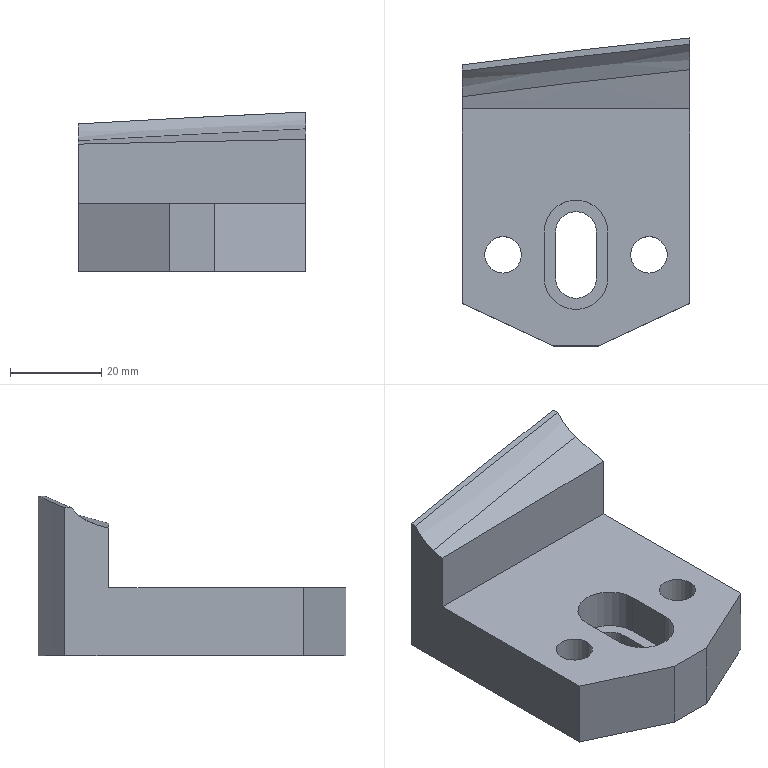Part | NX | features solid 2 | 1 solid | 23 faces | box 50 x 67.548 x 35.102 mm | volume 50758 mm3 | plane 13 | cylinder 6 | spline 4 | commonest cylinder face diameters 8 x2 9 x2 14 x2
STEP:
#1=CARTESIAN_POINT('',(-293.,-490.,-80.));
#2=VERTEX_POINT('',#1);
#3=CARTESIAN_POINT('',(-293.,-490.,-89.));
#4=VERTEX_POINT('',#3);
#5=CARTESIAN_POINT('',(-293.,-490.,-90.));
#6=DIRECTION('',(-0.000000149,0.000000502,1.));
#7=VECTOR('',#6,1000.);
#8=LINE('',#5,#7);
#9=EDGE_CURVE('',#2,#4,#8,.F.);
#10=ORIENTED_EDGE('',*,*,#9,.T.);
#11=CARTESIAN_POINT('',(-307.,-490.,-89.));
#12=VERTEX_POINT('',#11);
#13=CARTESIAN_POINT('',(-300.,-490.,-89.));
#14=DIRECTION('',(-0.000000149,0.000000502,1.));
#15=DIRECTION('',(0.,-1.,0.000000502));
#16=AXIS2_PLACEMENT_3D('',#13,#14,#15);
#17=CIRCLE('',#16,7.);
#18=EDGE_CURVE('',#12,#4,#17,.T.);
#19=ORIENTED_EDGE('',*,*,#18,.F.);
#20=CARTESIAN_POINT('',(-307.,-490.,-80.));
#21=VERTEX_POINT('',#20);
#22=CARTESIAN_POINT('',(-307.,-490.,-90.));
#23=DIRECTION('',(0.000000149,-0.000000502,-1.));
#24=VECTOR('',#23,1000.);
#25=LINE('',#22,#24);
#26=EDGE_CURVE('',#21,#12,#25,.T.);
#27=ORIENTED_EDGE('',*,*,#26,.F.);
#28=CARTESIAN_POINT('',(-300.,-490.,-80.));
#29=DIRECTION('',(0.000000149,-0.000000502,-1.));
#30=DIRECTION('',(0.,-1.,0.000000502));
#31=AXIS2_PLACEMENT_3D('',#28,#29,#30);
#32=CIRCLE('',#31,7.);
#33=EDGE_CURVE('',#2,#21,#32,.T.);
#34=ORIENTED_EDGE('',*,*,#33,.F.);
#35=EDGE_LOOP('',(#10,#19,#27,#34));
#36=FACE_BOUND('',#35,.T.);
#37=CARTESIAN_POINT('',(-300.,-490.,-90.));
#38=DIRECTION('',(0.000000149,-0.000000502,-1.));
#39=DIRECTION('',(1.,-0.000001668,0.000000149));
#40=AXIS2_PLACEMENT_3D('',#37,#38,#39);
#41=CYLINDRICAL_SURFACE('',#40,7.);
#42=ADVANCED_FACE('',(#36),#41,.F.);
#43=CARTESIAN_POINT('',(-293.,-480.,-80.));
#44=VERTEX_POINT('',#43);
#45=CARTESIAN_POINT('',(-293.,-480.,-89.));
#46=VERTEX_POINT('',#45);
#47=CARTESIAN_POINT('',(-293.,-480.,-90.));
#48=DIRECTION('',(0.000000149,-0.000000502,-1.));
#49=VECTOR('',#48,1000.);
#50=LINE('',#47,#49);
#51=EDGE_CURVE('',#44,#46,#50,.T.);
#52=ORIENTED_EDGE('',*,*,#51,.T.);
#53=CARTESIAN_POINT('',(-293.,-490.,-89.));
#54=DIRECTION('',(0.000001668,1.,-0.000000502));
#55=VECTOR('',#54,1000.);
#56=LINE('',#53,#55);
#57=EDGE_CURVE('',#4,#46,#56,.T.);
#58=ORIENTED_EDGE('',*,*,#57,.F.);
#59=ORIENTED_EDGE('',*,*,#9,.F.);
#60=CARTESIAN_POINT('',(-293.,-480.,-80.));
#61=DIRECTION('',(-0.000001668,-1.,0.000000502));
#62=VECTOR('',#61,1000.);
#63=LINE('',#60,#62);
#64=EDGE_CURVE('',#44,#2,#63,.T.);
#65=ORIENTED_EDGE('',*,*,#64,.F.);
#66=EDGE_LOOP('',(#52,#58,#59,#65));
#67=FACE_BOUND('',#66,.T.);
#68=CARTESIAN_POINT('',(-293.,-480.,-90.));
#69=DIRECTION('',(-1.,0.000001668,-0.000000149));
#70=DIRECTION('',(0.000001668,1.,-0.000000502));
#71=AXIS2_PLACEMENT_3D('',#68,#69,#70);
#72=PLANE('',#71);
#73=ADVANCED_FACE('',(#67),#72,.T.);
#74=CARTESIAN_POINT('',(-307.,-480.,-89.));
#75=VERTEX_POINT('',#74);
#76=CARTESIAN_POINT('',(-300.,-480.,-89.));
#77=DIRECTION('',(0.000000149,-0.000000502,-1.));
#78=DIRECTION('',(0.,-1.,0.000000502));
#79=AXIS2_PLACEMENT_3D('',#76,#77,#78);
#80=CIRCLE('',#79,7.);
#81=EDGE_CURVE('',#75,#46,#80,.T.);
#82=ORIENTED_EDGE('',*,*,#81,.T.);
#83=ORIENTED_EDGE('',*,*,#51,.F.);
#84=CARTESIAN_POINT('',(-307.,-480.,-80.));
#85=VERTEX_POINT('',#84);
#86=CARTESIAN_POINT('',(-300.,-480.,-80.));
#87=DIRECTION('',(0.000000149,-0.000000502,-1.));
#88=DIRECTION('',(0.,-1.,0.000000502));
#89=AXIS2_PLACEMENT_3D('',#86,#87,#88);
#90=CIRCLE('',#89,7.);
#91=EDGE_CURVE('',#44,#85,#90,.F.);
#92=ORIENTED_EDGE('',*,*,#91,.T.);
#93=CARTESIAN_POINT('',(-307.,-480.,-90.));
#94=DIRECTION('',(-0.000000149,0.000000502,1.));
#95=VECTOR('',#94,1000.);
#96=LINE('',#93,#95);
#97=EDGE_CURVE('',#85,#75,#96,.F.);
#98=ORIENTED_EDGE('',*,*,#97,.T.);
#99=EDGE_LOOP('',(#82,#83,#92,#98));
#100=FACE_BOUND('',#99,.T.);
#101=CARTESIAN_POINT('',(-300.,-480.,-90.));
#102=DIRECTION('',(0.000000149,-0.000000502,-1.));
#103=DIRECTION('',(1.,-0.000001668,0.000000149));
#104=AXIS2_PLACEMENT_3D('',#101,#102,#103);
#105=CYLINDRICAL_SURFACE('',#104,7.);
#106=ADVANCED_FACE('',(#100),#105,.F.);
#107=CARTESIAN_POINT('',(-307.,-490.,-89.));
#108=DIRECTION('',(0.000001668,1.,-0.000000502));
#109=VECTOR('',#108,1000.);
#110=LINE('',#107,#109);
#111=EDGE_CURVE('',#12,#75,#110,.T.);
#112=ORIENTED_EDGE('',*,*,#111,.T.);
#113=ORIENTED_EDGE('',*,*,#97,.F.);
#114=CARTESIAN_POINT('',(-307.,-480.,-80.));
#115=DIRECTION('',(-0.000001668,-1.,0.000000502));
#116=VECTOR('',#115,1000.);
#117=LINE('',#114,#116);
#118=EDGE_CURVE('',#85,#21,#117,.T.);
#119=ORIENTED_EDGE('',*,*,#118,.T.);
#120=ORIENTED_EDGE('',*,*,#26,.T.);
#121=EDGE_LOOP('',(#112,#113,#119,#120));
#122=FACE_BOUND('',#121,.T.);
#123=CARTESIAN_POINT('',(-307.,-480.,-90.));
#124=DIRECTION('',(-1.,0.000001668,-0.000000149));
#125=DIRECTION('',(0.000001668,1.,-0.000000502));
#126=AXIS2_PLACEMENT_3D('',#123,#124,#125);
#127=PLANE('',#126);
#128=ADVANCED_FACE('',(#122),#127,.F.);
#129=CARTESIAN_POINT('',(-275.,-437.456,-59.898));
#130=VERTEX_POINT('',#129);
#131=CARTESIAN_POINT('',(-275.,-437.453,-95.));
#132=VERTEX_POINT('',#131);
#133=CARTESIAN_POINT('',(-275.,-437.456,-59.898));
#134=CARTESIAN_POINT('',(-275.,-437.455,-71.599));
#135=CARTESIAN_POINT('',(-275.,-437.454,-83.299));
#136=CARTESIAN_POINT('',(-275.,-437.453,-95.));
#137=B_SPLINE_CURVE_WITH_KNOTS('',3,(#133,#134,#135,#136),.UNSPECIFIED.,.F.,.F.,(4,4),(-0.001705,0.0334),.UNSPECIFIED.);
#138=EDGE_CURVE('',#130,#132,#137,.T.);
#139=ORIENTED_EDGE('',*,*,#138,.T.);
#140=CARTESIAN_POINT('',(-325.,-443.348,-95.));
#141=VERTEX_POINT('',#140);
#142=CARTESIAN_POINT('',(-325.,-443.348,-95.));
#143=CARTESIAN_POINT('',(-308.358,-441.169,-95.));
#144=CARTESIAN_POINT('',(-291.693,-439.197,-95.));
#145=CARTESIAN_POINT('',(-275.,-437.453,-95.));
#146=B_SPLINE_CURVE_WITH_KNOTS('',3,(#142,#143,#144,#145),.UNSPECIFIED.,.F.,.F.,(4,4),(0.,0.05035),.UNSPECIFIED.);
#147=EDGE_CURVE('',#141,#132,#146,.T.);
#148=ORIENTED_EDGE('',*,*,#147,.F.);
#149=CARTESIAN_POINT('',(-325.,-443.347,-62.497));
#150=VERTEX_POINT('',#149);
#151=CARTESIAN_POINT('',(-325.,-443.347,-62.497));
#152=CARTESIAN_POINT('',(-325.,-443.348,-73.331));
#153=CARTESIAN_POINT('',(-325.,-443.348,-84.166));
#154=CARTESIAN_POINT('',(-325.,-443.348,-95.));
#155=B_SPLINE_CURVE_WITH_KNOTS('',3,(#151,#152,#153,#154),.UNSPECIFIED.,.F.,.F.,(4,4),(0.001175,0.03368),.UNSPECIFIED.);
#156=EDGE_CURVE('',#150,#141,#155,.T.);
#157=ORIENTED_EDGE('',*,*,#156,.F.);
#158=CARTESIAN_POINT('',(-275.,-437.456,-59.898));
#159=CARTESIAN_POINT('',(-291.695,-439.202,-60.667));
#160=CARTESIAN_POINT('',(-308.366,-441.17,-61.529));
#161=CARTESIAN_POINT('',(-325.,-443.347,-62.497));
#162=B_SPLINE_CURVE_WITH_KNOTS('',3,(#158,#159,#160,#161),.UNSPECIFIED.,.F.,.F.,(4,4),(0.3256,0.376),.UNSPECIFIED.);
#163=EDGE_CURVE('',#130,#150,#162,.T.);
#164=ORIENTED_EDGE('',*,*,#163,.F.);
#165=EDGE_LOOP('',(#139,#148,#157,#164));
#166=FACE_BOUND('',#165,.T.);
#167=CARTESIAN_POINT('',(-325.299,-443.386,-62.3));
#168=CARTESIAN_POINT('',(-325.3,-443.387,-74.142));
#169=CARTESIAN_POINT('',(-325.3,-443.387,-85.983));
#170=CARTESIAN_POINT('',(-325.3,-443.388,-97.824));
#171=CARTESIAN_POINT('',(-324.69,-443.307,-62.265));
#172=CARTESIAN_POINT('',(-324.691,-443.307,-74.106));
#173=CARTESIAN_POINT('',(-324.691,-443.307,-85.948));
#174=CARTESIAN_POINT('',(-324.691,-443.308,-97.789));
#175=CARTESIAN_POINT('',(-324.081,-443.227,-62.23));
#176=CARTESIAN_POINT('',(-324.082,-443.227,-74.071));
#177=CARTESIAN_POINT('',(-324.082,-443.228,-85.912));
#178=CARTESIAN_POINT('',(-324.082,-443.228,-97.754));
#179=CARTESIAN_POINT('',(-307.244,-441.038,-61.259));
#180=CARTESIAN_POINT('',(-307.244,-441.038,-73.1));
#181=CARTESIAN_POINT('',(-307.244,-441.037,-84.941));
#182=CARTESIAN_POINT('',(-307.244,-441.037,-96.783));
#183=CARTESIAN_POINT('',(-290.984,-439.125,-60.421));
#184=CARTESIAN_POINT('',(-290.984,-439.123,-72.262));
#185=CARTESIAN_POINT('',(-290.984,-439.122,-84.103));
#186=CARTESIAN_POINT('',(-290.984,-439.12,-95.944));
#187=CARTESIAN_POINT('',(-274.699,-437.425,-59.674));
#188=CARTESIAN_POINT('',(-274.699,-437.423,-71.515));
#189=CARTESIAN_POINT('',(-274.699,-437.422,-83.356));
#190=CARTESIAN_POINT('',(-274.699,-437.421,-95.197));
#191=B_SPLINE_SURFACE_WITH_KNOTS('',3,3,((#167,#168,#169,#170),(#171,#172,#173,#174),(#175,#176,#177,#178),(#179,#180,#181,#182),(#183,#184,#185,#186),(#187,#188,#189,#190)),.UNSPECIFIED.,.F.,.F.,.F.,(4,2,4),(4,4),(0.4571,0.4583,0.4899),(2.468,3.545),.UNSPECIFIED.);
#192=ADVANCED_FACE('',(#166),#191,.T.);
#193=ORIENTED_EDGE('',*,*,#156,.T.);
#194=CARTESIAN_POINT('',(-325.,-495.674,-95.));
#195=VERTEX_POINT('',#194);
#196=CARTESIAN_POINT('',(-325.,-453.,-95.));
#197=DIRECTION('',(-0.000001668,-1.,0.000000502));
#198=VECTOR('',#197,1000.);
#199=LINE('',#196,#198);
#200=EDGE_CURVE('',#141,#195,#199,.T.);
#201=ORIENTED_EDGE('',*,*,#200,.T.);
#202=CARTESIAN_POINT('',(-325.,-495.674,-80.));
#203=VERTEX_POINT('',#202);
#204=CARTESIAN_POINT('',(-325.,-495.674,-90.));
#205=DIRECTION('',(0.000000149,-0.000000502,-1.));
#206=VECTOR('',#205,1000.);
#207=LINE('',#204,#206);
#208=EDGE_CURVE('',#203,#195,#207,.T.);
#209=ORIENTED_EDGE('',*,*,#208,.F.);
#210=CARTESIAN_POINT('',(-325.,-453.,-80.));
#211=VERTEX_POINT('',#210);
#212=CARTESIAN_POINT('',(-325.,-453.,-80.));
#213=DIRECTION('',(-0.000001668,-1.,0.000000502));
#214=VECTOR('',#213,1000.);
#215=LINE('',#212,#214);
#216=EDGE_CURVE('',#211,#203,#215,.T.);
#217=ORIENTED_EDGE('',*,*,#216,.F.);
#218=CARTESIAN_POINT('',(-325.,-453.,-66.946));
#219=VERTEX_POINT('',#218);
#220=CARTESIAN_POINT('',(-325.,-453.,-105.));
#221=DIRECTION('',(-0.000000149,0.000000502,1.));
#222=VECTOR('',#221,1000.);
#223=LINE('',#220,#222);
#224=EDGE_CURVE('',#219,#211,#223,.F.);
#225=ORIENTED_EDGE('',*,*,#224,.F.);
#226=CARTESIAN_POINT('',(-325.,-450.324,-66.214));
#227=VERTEX_POINT('',#226);
#228=CARTESIAN_POINT('',(-325.,-453.,-66.946));
#229=CARTESIAN_POINT('',(-325.,-452.108,-66.702));
#230=CARTESIAN_POINT('',(-325.,-451.216,-66.458));
#231=CARTESIAN_POINT('',(-325.,-450.324,-66.215));
#232=B_SPLINE_CURVE_WITH_KNOTS('',3,(#228,#229,#230,#231),.UNSPECIFIED.,.F.,.F.,(4,4),(0.01659,0.01936),.UNSPECIFIED.);
#233=EDGE_CURVE('',#219,#227,#232,.T.);
#234=ORIENTED_EDGE('',*,*,#233,.T.);
#235=CARTESIAN_POINT('',(-325.,-444.724,-62.497));
#236=VERTEX_POINT('',#235);
#237=CARTESIAN_POINT('',(-325.,-450.324,-66.214));
#238=CARTESIAN_POINT('',(-325.,-448.107,-65.608));
#239=CARTESIAN_POINT('',(-325.,-446.142,-64.306));
#240=CARTESIAN_POINT('',(-325.,-444.724,-62.497));
#241=B_SPLINE_CURVE_WITH_KNOTS('',3,(#237,#238,#239,#240),.UNSPECIFIED.,.F.,.F.,(4,4),(0.,0.006804),.UNSPECIFIED.);
#242=EDGE_CURVE('',#227,#236,#241,.T.);
#243=ORIENTED_EDGE('',*,*,#242,.T.);
#244=CARTESIAN_POINT('',(-325.,-443.347,-62.497));
#245=CARTESIAN_POINT('',(-325.,-443.806,-62.497));
#246=CARTESIAN_POINT('',(-325.,-444.265,-62.497));
#247=CARTESIAN_POINT('',(-325.,-444.724,-62.497));
#248=B_SPLINE_CURVE_WITH_KNOTS('',3,(#244,#245,#246,#247),.UNSPECIFIED.,.F.,.F.,(4,4),(0.,0.001377),.UNSPECIFIED.);
#249=EDGE_CURVE('',#150,#236,#248,.T.);
#250=ORIENTED_EDGE('',*,*,#249,.F.);
#251=EDGE_LOOP('',(#193,#201,#209,#217,#225,#234,#243,#250));
#252=FACE_BOUND('',#251,.T.);
#253=CARTESIAN_POINT('',(-325.,-453.,-90.));
#254=DIRECTION('',(-1.,0.000001668,-0.000000149));
#255=DIRECTION('',(0.000001668,1.,-0.000000502));
#256=AXIS2_PLACEMENT_3D('',#253,#254,#255);
#257=PLANE('',#256);
#258=ADVANCED_FACE('',(#252),#257,.T.);
#259=CARTESIAN_POINT('',(-275.,-438.851,-59.898));
#260=VERTEX_POINT('',#259);
#261=CARTESIAN_POINT('',(-275.,-437.456,-59.898));
#262=CARTESIAN_POINT('',(-275.,-437.921,-59.898));
#263=CARTESIAN_POINT('',(-275.,-438.386,-59.898));
#264=CARTESIAN_POINT('',(-275.,-438.851,-59.898));
#265=B_SPLINE_CURVE_WITH_KNOTS('',3,(#261,#262,#263,#264),.UNSPECIFIED.,.F.,.F.,(4,4),(0.009864,0.01126),.UNSPECIFIED.);
#266=EDGE_CURVE('',#130,#260,#265,.T.);
#267=ORIENTED_EDGE('',*,*,#266,.T.);
#268=CARTESIAN_POINT('',(-275.,-444.433,-63.598));
#269=VERTEX_POINT('',#268);
#270=CARTESIAN_POINT('',(-275.,-444.433,-63.598));
#271=CARTESIAN_POINT('',(-275.,-442.223,-62.998));
#272=CARTESIAN_POINT('',(-275.,-440.264,-61.702));
#273=CARTESIAN_POINT('',(-275.,-438.851,-59.898));
#274=B_SPLINE_CURVE_WITH_KNOTS('',3,(#270,#271,#272,#273),.UNSPECIFIED.,.F.,.F.,(4,4),(0.,0.006779),.UNSPECIFIED.);
#275=EDGE_CURVE('',#269,#260,#274,.T.);
#276=ORIENTED_EDGE('',*,*,#275,.F.);
#277=CARTESIAN_POINT('',(-275.,-453.,-65.922));
#278=VERTEX_POINT('',#277);
#279=CARTESIAN_POINT('',(-275.,-453.,-65.922));
#280=CARTESIAN_POINT('',(-275.,-450.144,-65.148));
#281=CARTESIAN_POINT('',(-275.,-447.289,-64.373));
#282=CARTESIAN_POINT('',(-275.,-444.433,-63.599));
#283=B_SPLINE_CURVE_WITH_KNOTS('',3,(#279,#280,#281,#282),.UNSPECIFIED.,.F.,.F.,(4,4),(0.,0.008876),.UNSPECIFIED.);
#284=EDGE_CURVE('',#278,#269,#283,.T.);
#285=ORIENTED_EDGE('',*,*,#284,.F.);
#286=CARTESIAN_POINT('',(-275.,-453.,-80.));
#287=VERTEX_POINT('',#286);
#288=CARTESIAN_POINT('',(-275.,-453.,-105.));
#289=DIRECTION('',(-0.000000149,0.000000502,1.));
#290=VECTOR('',#289,1000.);
#291=LINE('',#288,#290);
#292=EDGE_CURVE('',#278,#287,#291,.F.);
#293=ORIENTED_EDGE('',*,*,#292,.T.);
#294=CARTESIAN_POINT('',(-275.,-495.674,-80.));
#295=VERTEX_POINT('',#294);
#296=CARTESIAN_POINT('',(-275.,-445.,-80.));
#297=DIRECTION('',(-0.000001668,-1.,0.000000502));
#298=VECTOR('',#297,1000.);
#299=LINE('',#296,#298);
#300=EDGE_CURVE('',#287,#295,#299,.T.);
#301=ORIENTED_EDGE('',*,*,#300,.T.);
#302=CARTESIAN_POINT('',(-275.,-495.674,-95.));
#303=VERTEX_POINT('',#302);
#304=CARTESIAN_POINT('',(-275.,-495.674,-90.));
#305=DIRECTION('',(0.000000149,-0.000000502,-1.));
#306=VECTOR('',#305,1000.);
#307=LINE('',#304,#306);
#308=EDGE_CURVE('',#295,#303,#307,.T.);
#309=ORIENTED_EDGE('',*,*,#308,.T.);
#310=CARTESIAN_POINT('',(-275.,-445.,-95.));
#311=DIRECTION('',(-0.000001668,-1.,0.000000502));
#312=VECTOR('',#311,1000.);
#313=LINE('',#310,#312);
#314=EDGE_CURVE('',#132,#303,#313,.T.);
#315=ORIENTED_EDGE('',*,*,#314,.F.);
#316=ORIENTED_EDGE('',*,*,#138,.F.);
#317=EDGE_LOOP('',(#267,#276,#285,#293,#301,#309,#315,#316));
#318=FACE_BOUND('',#317,.T.);
#319=CARTESIAN_POINT('',(-275.,-445.,-90.));
#320=DIRECTION('',(-1.,0.000001668,-0.000000149));
#321=DIRECTION('',(0.000000149,-0.000000502,-1.));
#322=AXIS2_PLACEMENT_3D('',#319,#320,#321);
#323=PLANE('',#322);
#324=ADVANCED_FACE('',(#318),#323,.F.);
#325=ORIENTED_EDGE('',*,*,#200,.F.);
#326=ORIENTED_EDGE('',*,*,#147,.T.);
#327=ORIENTED_EDGE('',*,*,#314,.T.);
#328=CARTESIAN_POINT('',(-295.,-505.,-95.));
#329=VERTEX_POINT('',#328);
#330=CARTESIAN_POINT('',(-275.,-495.674,-95.));
#331=DIRECTION('',(-0.9063,-0.4226,0.000000077));
#332=VECTOR('',#331,1000.);
#333=LINE('',#330,#332);
#334=EDGE_CURVE('',#303,#329,#333,.T.);
#335=ORIENTED_EDGE('',*,*,#334,.T.);
#336=CARTESIAN_POINT('',(-305.,-505.,-95.));
#337=VERTEX_POINT('',#336);
#338=CARTESIAN_POINT('',(-295.,-505.,-95.));
#339=DIRECTION('',(-1.,0.000001668,-0.000000149));
#340=VECTOR('',#339,1000.);
#341=LINE('',#338,#340);
#342=EDGE_CURVE('',#329,#337,#341,.T.);
#343=ORIENTED_EDGE('',*,*,#342,.T.);
#344=CARTESIAN_POINT('',(-325.,-495.674,-95.));
#345=DIRECTION('',(0.9063,-0.4226,0.000000347));
#346=VECTOR('',#345,1000.);
#347=LINE('',#344,#346);
#348=EDGE_CURVE('',#195,#337,#347,.T.);
#349=ORIENTED_EDGE('',*,*,#348,.F.);
#350=EDGE_LOOP('',(#325,#326,#327,#335,#343,#349));
#351=FACE_BOUND('',#350,.T.);
#352=CARTESIAN_POINT('',(-316.,-489.,-95.));
#353=VERTEX_POINT('',#352);
#354=CARTESIAN_POINT('',(-316.,-485.,-95.));
#355=DIRECTION('',(0.000000149,-0.000000502,-1.));
#356=DIRECTION('',(0.,-1.,0.000000502));
#357=AXIS2_PLACEMENT_3D('',#354,#355,#356);
#358=CIRCLE('',#357,4.);
#359=EDGE_CURVE('',#353,#353,#358,.F.);
#360=ORIENTED_EDGE('',*,*,#359,.T.);
#361=EDGE_LOOP('',(#360));
#362=FACE_BOUND('',#361,.T.);
#363=CARTESIAN_POINT('',(-284.,-489.,-95.));
#364=VERTEX_POINT('',#363);
#365=CARTESIAN_POINT('',(-284.,-485.,-95.));
#366=DIRECTION('',(0.000000149,-0.000000502,-1.));
#367=DIRECTION('',(0.,-1.,0.000000502));
#368=AXIS2_PLACEMENT_3D('',#365,#366,#367);
#369=CIRCLE('',#368,4.);
#370=EDGE_CURVE('',#364,#364,#369,.F.);
#371=ORIENTED_EDGE('',*,*,#370,.T.);
#372=EDGE_LOOP('',(#371));
#373=FACE_BOUND('',#372,.T.);
#374=CARTESIAN_POINT('',(-304.5,-480.,-95.));
#375=VERTEX_POINT('',#374);
#376=CARTESIAN_POINT('',(-295.5,-480.,-95.));
#377=VERTEX_POINT('',#376);
#378=CARTESIAN_POINT('',(-300.,-480.,-95.));
#379=DIRECTION('',(0.000000149,-0.000000502,-1.));
#380=DIRECTION('',(0.,-1.,0.000000502));
#381=AXIS2_PLACEMENT_3D('',#378,#379,#380);
#382=CIRCLE('',#381,4.5);
#383=EDGE_CURVE('',#375,#377,#382,.T.);
#384=ORIENTED_EDGE('',*,*,#383,.F.);
#385=CARTESIAN_POINT('',(-304.5,-490.,-95.));
#386=VERTEX_POINT('',#385);
#387=CARTESIAN_POINT('',(-304.5,-480.,-95.));
#388=DIRECTION('',(-0.000001668,-1.,0.000000502));
#389=VECTOR('',#388,1000.);
#390=LINE('',#387,#389);
#391=EDGE_CURVE('',#375,#386,#390,.T.);
#392=ORIENTED_EDGE('',*,*,#391,.T.);
#393=CARTESIAN_POINT('',(-295.5,-490.,-95.));
#394=VERTEX_POINT('',#393);
#395=CARTESIAN_POINT('',(-300.,-490.,-95.));
#396=DIRECTION('',(0.000000149,-0.000000502,-1.));
#397=DIRECTION('',(0.,-1.,0.000000502));
#398=AXIS2_PLACEMENT_3D('',#395,#396,#397);
#399=CIRCLE('',#398,4.5);
#400=EDGE_CURVE('',#394,#386,#399,.T.);
#401=ORIENTED_EDGE('',*,*,#400,.F.);
#402=CARTESIAN_POINT('',(-295.5,-480.,-95.));
#403=DIRECTION('',(-0.000001668,-1.,0.000000502));
#404=VECTOR('',#403,1000.);
#405=LINE('',#402,#404);
#406=EDGE_CURVE('',#377,#394,#405,.T.);
#407=ORIENTED_EDGE('',*,*,#406,.F.);
#408=EDGE_LOOP('',(#384,#392,#401,#407));
#409=FACE_BOUND('',#408,.T.);
#410=CARTESIAN_POINT('',(-325.,-445.,-95.));
#411=DIRECTION('',(0.000000149,-0.000000502,-1.));
#412=DIRECTION('',(1.,-0.000001668,0.000000149));
#413=AXIS2_PLACEMENT_3D('',#410,#411,#412);
#414=PLANE('',#413);
#415=ADVANCED_FACE('',(#351,#362,#373,#409),#414,.T.);
#416=CARTESIAN_POINT('',(-325.,-453.,-66.946));
#417=CARTESIAN_POINT('',(-308.425,-453.,-66.568));
#418=CARTESIAN_POINT('',(-291.758,-453.,-66.227));
#419=CARTESIAN_POINT('',(-275.,-453.,-65.922));
#420=B_SPLINE_CURVE_WITH_KNOTS('',3,(#416,#417,#418,#419),.UNSPECIFIED.,.F.,.F.,(4,4),(0.,1.),.UNSPECIFIED.);
#421=EDGE_CURVE('',#278,#219,#420,.F.);
#422=ORIENTED_EDGE('',*,*,#421,.T.);
#423=ORIENTED_EDGE('',*,*,#224,.T.);
#424=CARTESIAN_POINT('',(-325.,-453.,-80.));
#425=DIRECTION('',(-1.,0.000001668,-0.000000149));
#426=VECTOR('',#425,1000.);
#427=LINE('',#424,#426);
#428=EDGE_CURVE('',#211,#287,#427,.F.);
#429=ORIENTED_EDGE('',*,*,#428,.T.);
#430=ORIENTED_EDGE('',*,*,#292,.F.);
#431=EDGE_LOOP('',(#422,#423,#429,#430));
#432=FACE_BOUND('',#431,.T.);
#433=CARTESIAN_POINT('',(-325.,-453.,-105.));
#434=DIRECTION('',(0.000001668,1.,-0.000000502));
#435=DIRECTION('',(1.,-0.000001668,0.000000149));
#436=AXIS2_PLACEMENT_3D('',#433,#434,#435);
#437=PLANE('',#436);
#438=ADVANCED_FACE('',(#432),#437,.F.);
#439=CARTESIAN_POINT('',(-316.,-489.,-80.));
#440=VERTEX_POINT('',#439);
#441=CARTESIAN_POINT('',(-316.,-485.,-80.));
#442=DIRECTION('',(0.000000149,-0.000000502,-1.));
#443=DIRECTION('',(0.,-1.,0.000000502));
#444=AXIS2_PLACEMENT_3D('',#441,#442,#443);
#445=CIRCLE('',#444,4.);
#446=EDGE_CURVE('',#440,#440,#445,.F.);
#447=ORIENTED_EDGE('',*,*,#446,.F.);
#448=EDGE_LOOP('',(#447));
#449=FACE_BOUND('',#448,.T.);
#450=CARTESIAN_POINT('',(-284.,-489.,-80.));
#451=VERTEX_POINT('',#450);
#452=CARTESIAN_POINT('',(-284.,-485.,-80.));
#453=DIRECTION('',(0.000000149,-0.000000502,-1.));
#454=DIRECTION('',(0.,-1.,0.000000502));
#455=AXIS2_PLACEMENT_3D('',#452,#453,#454);
#456=CIRCLE('',#455,4.);
#457=EDGE_CURVE('',#451,#451,#456,.F.);
#458=ORIENTED_EDGE('',*,*,#457,.F.);
#459=EDGE_LOOP('',(#458));
#460=FACE_BOUND('',#459,.T.);
#461=ORIENTED_EDGE('',*,*,#216,.T.);
#462=CARTESIAN_POINT('',(-305.,-505.,-80.));
#463=VERTEX_POINT('',#462);
#464=CARTESIAN_POINT('',(-325.,-495.674,-80.));
#465=DIRECTION('',(0.9063,-0.4226,0.000000347));
#466=VECTOR('',#465,1000.);
#467=LINE('',#464,#466);
#468=EDGE_CURVE('',#203,#463,#467,.T.);
#469=ORIENTED_EDGE('',*,*,#468,.T.);
#470=CARTESIAN_POINT('',(-295.,-505.,-80.));
#471=VERTEX_POINT('',#470);
#472=CARTESIAN_POINT('',(-295.,-505.,-80.));
#473=DIRECTION('',(-1.,0.000001668,-0.000000149));
#474=VECTOR('',#473,1000.);
#475=LINE('',#472,#474);
#476=EDGE_CURVE('',#471,#463,#475,.T.);
#477=ORIENTED_EDGE('',*,*,#476,.F.);
#478=CARTESIAN_POINT('',(-275.,-495.674,-80.));
#479=DIRECTION('',(-0.9063,-0.4226,0.000000077));
#480=VECTOR('',#479,1000.);
#481=LINE('',#478,#480);
#482=EDGE_CURVE('',#295,#471,#481,.T.);
#483=ORIENTED_EDGE('',*,*,#482,.F.);
#484=ORIENTED_EDGE('',*,*,#300,.F.);
#485=ORIENTED_EDGE('',*,*,#428,.F.);
#486=EDGE_LOOP('',(#461,#469,#477,#483,#484,#485));
#487=FACE_BOUND('',#486,.T.);
#488=ORIENTED_EDGE('',*,*,#33,.T.);
#489=ORIENTED_EDGE('',*,*,#118,.F.);
#490=ORIENTED_EDGE('',*,*,#91,.F.);
#491=ORIENTED_EDGE('',*,*,#64,.T.);
#492=EDGE_LOOP('',(#488,#489,#490,#491));
#493=FACE_BOUND('',#492,.T.);
#494=CARTESIAN_POINT('',(-325.,-445.,-80.));
#495=DIRECTION('',(0.000000149,-0.000000502,-1.));
#496=DIRECTION('',(1.,-0.000001668,0.000000149));
#497=AXIS2_PLACEMENT_3D('',#494,#495,#496);
#498=PLANE('',#497);
#499=ADVANCED_FACE('',(#449,#460,#487,#493),#498,.F.);
#500=ORIENTED_EDGE('',*,*,#348,.T.);
#501=CARTESIAN_POINT('',(-305.,-505.,-90.));
#502=DIRECTION('',(0.000000149,-0.000000502,-1.));
#503=VECTOR('',#502,1000.);
#504=LINE('',#501,#503);
#505=EDGE_CURVE('',#463,#337,#504,.T.);
#506=ORIENTED_EDGE('',*,*,#505,.F.);
#507=ORIENTED_EDGE('',*,*,#468,.F.);
#508=ORIENTED_EDGE('',*,*,#208,.T.);
#509=EDGE_LOOP('',(#500,#506,#507,#508));
#510=FACE_BOUND('',#509,.T.);
#511=CARTESIAN_POINT('',(-325.,-495.674,-90.));
#512=DIRECTION('',(-0.4226,-0.9063,0.000000392));
#513=DIRECTION('',(-0.9063,0.4226,-0.000000347));
#514=AXIS2_PLACEMENT_3D('',#511,#512,#513);
#515=PLANE('',#514);
#516=ADVANCED_FACE('',(#510),#515,.T.);
#517=ORIENTED_EDGE('',*,*,#342,.F.);
#518=CARTESIAN_POINT('',(-295.,-505.,-90.));
#519=DIRECTION('',(0.000000149,-0.000000502,-1.));
#520=VECTOR('',#519,1000.);
#521=LINE('',#518,#520);
#522=EDGE_CURVE('',#471,#329,#521,.T.);
#523=ORIENTED_EDGE('',*,*,#522,.F.);
#524=ORIENTED_EDGE('',*,*,#476,.T.);
#525=ORIENTED_EDGE('',*,*,#505,.T.);
#526=EDGE_LOOP('',(#517,#523,#524,#525));
#527=FACE_BOUND('',#526,.T.);
#528=CARTESIAN_POINT('',(-295.,-505.,-90.));
#529=DIRECTION('',(0.000001668,1.,-0.000000502));
#530=DIRECTION('',(-0.000000149,0.000000502,1.));
#531=AXIS2_PLACEMENT_3D('',#528,#529,#530);
#532=PLANE('',#531);
#533=ADVANCED_FACE('',(#527),#532,.F.);
#534=ORIENTED_EDGE('',*,*,#334,.F.);
#535=ORIENTED_EDGE('',*,*,#308,.F.);
#536=ORIENTED_EDGE('',*,*,#482,.T.);
#537=ORIENTED_EDGE('',*,*,#522,.T.);
#538=EDGE_LOOP('',(#534,#535,#536,#537));
#539=FACE_BOUND('',#538,.T.);
#540=CARTESIAN_POINT('',(-275.,-495.674,-90.));
#541=DIRECTION('',(-0.4226,0.9063,-0.000000518));
#542=DIRECTION('',(0.9063,0.4226,-0.000000077));
#543=AXIS2_PLACEMENT_3D('',#540,#541,#542);
#544=PLANE('',#543);
#545=ADVANCED_FACE('',(#539),#544,.F.);
#546=ORIENTED_EDGE('',*,*,#370,.F.);
#547=EDGE_LOOP('',(#546));
#548=FACE_BOUND('',#547,.T.);
#549=ORIENTED_EDGE('',*,*,#457,.T.);
#550=EDGE_LOOP('',(#549));
#551=FACE_BOUND('',#550,.T.);
#552=CARTESIAN_POINT('',(-284.,-485.,-90.));
#553=DIRECTION('',(0.000000149,-0.000000502,-1.));
#554=DIRECTION('',(1.,-0.000001668,0.000000149));
#555=AXIS2_PLACEMENT_3D('',#552,#553,#554);
#556=CYLINDRICAL_SURFACE('',#555,4.);
#557=ADVANCED_FACE('',(#548,#551),#556,.F.);
#558=ORIENTED_EDGE('',*,*,#359,.F.);
#559=EDGE_LOOP('',(#558));
#560=FACE_BOUND('',#559,.T.);
#561=ORIENTED_EDGE('',*,*,#446,.T.);
#562=EDGE_LOOP('',(#561));
#563=FACE_BOUND('',#562,.T.);
#564=CARTESIAN_POINT('',(-316.,-485.,-90.));
#565=DIRECTION('',(0.000000149,-0.000000502,-1.));
#566=DIRECTION('',(1.,-0.000001668,0.000000149));
#567=AXIS2_PLACEMENT_3D('',#564,#565,#566);
#568=CYLINDRICAL_SURFACE('',#567,4.);
#569=ADVANCED_FACE('',(#560,#563),#568,.F.);
#570=ORIENTED_EDGE('',*,*,#242,.F.);
#571=CARTESIAN_POINT('',(-325.,-450.324,-66.214));
#572=CARTESIAN_POINT('',(-308.365,-448.137,-65.24));
#573=CARTESIAN_POINT('',(-291.697,-446.183,-64.372));
#574=CARTESIAN_POINT('',(-275.,-444.433,-63.598));
#575=B_SPLINE_CURVE_WITH_KNOTS('',3,(#571,#572,#573,#574),.UNSPECIFIED.,.F.,.F.,(4,4),(0.3691,0.4667),.UNSPECIFIED.);
#576=EDGE_CURVE('',#269,#227,#575,.F.);
#577=ORIENTED_EDGE('',*,*,#576,.F.);
#578=ORIENTED_EDGE('',*,*,#275,.T.);
#579=CARTESIAN_POINT('',(-325.,-444.724,-62.497));
#580=CARTESIAN_POINT('',(-308.365,-442.543,-61.529));
#581=CARTESIAN_POINT('',(-291.696,-440.596,-60.667));
#582=CARTESIAN_POINT('',(-275.,-438.851,-59.898));
#583=B_SPLINE_CURVE_WITH_KNOTS('',3,(#579,#580,#581,#582),.UNSPECIFIED.,.F.,.F.,(4,4),(0.,0.05041),.UNSPECIFIED.);
#584=EDGE_CURVE('',#236,#260,#583,.T.);
#585=ORIENTED_EDGE('',*,*,#584,.F.);
#586=EDGE_LOOP('',(#570,#577,#578,#585));
#587=FACE_BOUND('',#586,.T.);
#588=CARTESIAN_POINT('',(-273.95,-444.324,-63.55));
#589=CARTESIAN_POINT('',(-274.346,-440.936,-62.638));
#590=CARTESIAN_POINT('',(-274.698,-438.794,-59.852));
#591=CARTESIAN_POINT('',(-291.099,-446.112,-64.34));
#592=CARTESIAN_POINT('',(-291.528,-442.728,-63.428));
#593=CARTESIAN_POINT('',(-291.908,-440.59,-60.643));
#594=CARTESIAN_POINT('',(-308.219,-448.115,-65.23));
#595=CARTESIAN_POINT('',(-308.681,-444.734,-64.318));
#596=CARTESIAN_POINT('',(-309.093,-442.601,-61.533));
#597=CARTESIAN_POINT('',(-325.304,-450.364,-66.232));
#598=CARTESIAN_POINT('',(-325.803,-446.989,-65.321));
#599=CARTESIAN_POINT('',(-326.247,-444.862,-62.537));
#600=(BOUNDED_SURFACE()B_SPLINE_SURFACE(3,2,((#588,#589,#590),(#591,#592,#593),(#594,#595,#596),(#597,#598,#599)),.UNSPECIFIED.,.F.,.F.,.F.)B_SPLINE_SURFACE_WITH_KNOTS((4,4),(3,3),(0.3008,0.3527),(0.,0.969),.PIECEWISE_BEZIER_KNOTS.)GEOMETRIC_REPRESENTATION_ITEM()RATIONAL_B_SPLINE_SURFACE(((1.,0.9463,0.9967),(1.,0.9463,0.9967),(1.,0.9462,0.9967),(1.,0.9462,0.9967)))REPRESENTATION_ITEM('')SURFACE());
#601=ADVANCED_FACE('',(#587),#600,.F.);
#602=ORIENTED_EDGE('',*,*,#233,.F.);
#603=ORIENTED_EDGE('',*,*,#421,.F.);
#604=ORIENTED_EDGE('',*,*,#284,.T.);
#605=ORIENTED_EDGE('',*,*,#576,.T.);
#606=EDGE_LOOP('',(#602,#603,#604,#605));
#607=FACE_BOUND('',#606,.T.);
#608=CARTESIAN_POINT('',(-274.704,-444.351,-63.571));
#609=CARTESIAN_POINT('',(-274.274,-447.196,-64.335));
#610=CARTESIAN_POINT('',(-273.843,-450.041,-65.099));
#611=CARTESIAN_POINT('',(-273.413,-452.886,-65.863));
#612=CARTESIAN_POINT('',(-291.763,-446.131,-64.358));
#613=CARTESIAN_POINT('',(-291.306,-448.969,-65.121));
#614=CARTESIAN_POINT('',(-290.848,-451.808,-65.883));
#615=CARTESIAN_POINT('',(-290.391,-454.647,-66.646));
#616=CARTESIAN_POINT('',(-308.79,-448.139,-65.25));
#617=CARTESIAN_POINT('',(-308.305,-450.975,-66.012));
#618=CARTESIAN_POINT('',(-307.82,-453.812,-66.775));
#619=CARTESIAN_POINT('',(-307.335,-456.649,-67.537));
#620=CARTESIAN_POINT('',(-325.783,-450.375,-66.246));
#621=CARTESIAN_POINT('',(-325.27,-453.214,-67.01));
#622=CARTESIAN_POINT('',(-324.757,-456.053,-67.774));
#623=CARTESIAN_POINT('',(-324.244,-458.892,-68.538));
#624=B_SPLINE_SURFACE_WITH_KNOTS('',3,3,((#608,#609,#610,#611),(#612,#613,#614,#615),(#616,#617,#618,#619),(#620,#621,#622,#623)),.UNSPECIFIED.,.F.,.F.,.F.,(4,4),(4,4),(0.5328,0.6325),(-0.00122,0.204),.UNSPECIFIED.);
#625=ADVANCED_FACE('',(#607),#624,.T.);
#626=ORIENTED_EDGE('',*,*,#163,.T.);
#627=ORIENTED_EDGE('',*,*,#249,.T.);
#628=ORIENTED_EDGE('',*,*,#584,.T.);
#629=ORIENTED_EDGE('',*,*,#266,.F.);
#630=EDGE_LOOP('',(#626,#627,#628,#629));
#631=FACE_BOUND('',#630,.T.);
#632=CARTESIAN_POINT('',(-325.299,-443.361,-62.514));
#633=CARTESIAN_POINT('',(-325.299,-444.773,-62.514));
#634=CARTESIAN_POINT('',(-308.461,-441.151,-61.533));
#635=CARTESIAN_POINT('',(-308.461,-442.562,-61.533));
#636=CARTESIAN_POINT('',(-291.593,-439.18,-60.661));
#637=CARTESIAN_POINT('',(-291.593,-440.591,-60.661));
#638=CARTESIAN_POINT('',(-274.699,-437.416,-59.884));
#639=CARTESIAN_POINT('',(-274.699,-438.828,-59.884));
#640=B_SPLINE_SURFACE_WITH_KNOTS('',3,1,((#632,#633),(#634,#635),(#636,#637),(#638,#639)),.SURF_OF_LINEAR_EXTRUSION.,.F.,.F.,.F.,(4,4),(2,2),(-0.006578,1.006),(0.,1.),.PIECEWISE_BEZIER_KNOTS.);
#641=ADVANCED_FACE('',(#631),#640,.F.);
#642=CARTESIAN_POINT('',(-304.5,-480.,-89.));
#643=VERTEX_POINT('',#642);
#644=CARTESIAN_POINT('',(-304.5,-490.,-89.));
#645=VERTEX_POINT('',#644);
#646=CARTESIAN_POINT('',(-304.5,-480.,-89.));
#647=DIRECTION('',(-0.000001668,-1.,0.000000502));
#648=VECTOR('',#647,1000.);
#649=LINE('',#646,#648);
#650=EDGE_CURVE('',#643,#645,#649,.T.);
#651=ORIENTED_EDGE('',*,*,#650,.F.);
#652=CARTESIAN_POINT('',(-295.5,-480.,-89.));
#653=VERTEX_POINT('',#652);
#654=CARTESIAN_POINT('',(-300.,-480.,-89.));
#655=DIRECTION('',(0.000000149,-0.000000502,-1.));
#656=DIRECTION('',(0.,-1.,0.000000502));
#657=AXIS2_PLACEMENT_3D('',#654,#655,#656);
#658=CIRCLE('',#657,4.5);
#659=EDGE_CURVE('',#643,#653,#658,.T.);
#660=ORIENTED_EDGE('',*,*,#659,.T.);
#661=CARTESIAN_POINT('',(-295.5,-490.,-89.));
#662=VERTEX_POINT('',#661);
#663=CARTESIAN_POINT('',(-295.5,-480.,-89.));
#664=DIRECTION('',(-0.000001668,-1.,0.000000502));
#665=VECTOR('',#664,1000.);
#666=LINE('',#663,#665);
#667=EDGE_CURVE('',#653,#662,#666,.T.);
#668=ORIENTED_EDGE('',*,*,#667,.T.);
#669=CARTESIAN_POINT('',(-300.,-490.,-89.));
#670=DIRECTION('',(0.000000149,-0.000000502,-1.));
#671=DIRECTION('',(0.,-1.,0.000000502));
#672=AXIS2_PLACEMENT_3D('',#669,#670,#671);
#673=CIRCLE('',#672,4.5);
#674=EDGE_CURVE('',#662,#645,#673,.T.);
#675=ORIENTED_EDGE('',*,*,#674,.T.);
#676=EDGE_LOOP('',(#651,#660,#668,#675));
#677=FACE_BOUND('',#676,.T.);
#678=ORIENTED_EDGE('',*,*,#81,.F.);
#679=ORIENTED_EDGE('',*,*,#111,.F.);
#680=ORIENTED_EDGE('',*,*,#18,.T.);
#681=ORIENTED_EDGE('',*,*,#57,.T.);
#682=EDGE_LOOP('',(#678,#679,#680,#681));
#683=FACE_BOUND('',#682,.T.);
#684=CARTESIAN_POINT('',(-300.,-480.,-89.));
#685=DIRECTION('',(0.000000149,-0.000000502,-1.));
#686=DIRECTION('',(0.,-1.,0.000000502));
#687=AXIS2_PLACEMENT_3D('',#684,#685,#686);
#688=PLANE('',#687);
#689=ADVANCED_FACE('',(#677,#683),#688,.F.);
#690=CARTESIAN_POINT('',(-304.5,-480.,-180.));
#691=DIRECTION('',(0.,0.,1.));
#692=VECTOR('',#691,1000.);
#693=LINE('',#690,#692);
#694=EDGE_CURVE('',#375,#643,#693,.T.);
#695=ORIENTED_EDGE('',*,*,#694,.F.);
#696=ORIENTED_EDGE('',*,*,#383,.T.);
#697=CARTESIAN_POINT('',(-295.5,-480.,-180.));
#698=DIRECTION('',(0.,0.,1.));
#699=VECTOR('',#698,1000.);
#700=LINE('',#697,#699);
#701=EDGE_CURVE('',#377,#653,#700,.T.);
#702=ORIENTED_EDGE('',*,*,#701,.T.);
#703=ORIENTED_EDGE('',*,*,#659,.F.);
#704=EDGE_LOOP('',(#695,#696,#702,#703));
#705=FACE_BOUND('',#704,.T.);
#706=CARTESIAN_POINT('',(-300.,-480.,-180.));
#707=DIRECTION('',(0.,0.,1.));
#708=DIRECTION('',(0.,1.,0.));
#709=AXIS2_PLACEMENT_3D('',#706,#707,#708);
#710=CYLINDRICAL_SURFACE('',#709,4.5);
#711=ADVANCED_FACE('',(#705),#710,.F.);
#712=ORIENTED_EDGE('',*,*,#650,.T.);
#713=CARTESIAN_POINT('',(-304.5,-490.,-180.));
#714=DIRECTION('',(0.,0.,1.));
#715=VECTOR('',#714,1000.);
#716=LINE('',#713,#715);
#717=EDGE_CURVE('',#386,#645,#716,.T.);
#718=ORIENTED_EDGE('',*,*,#717,.F.);
#719=ORIENTED_EDGE('',*,*,#391,.F.);
#720=ORIENTED_EDGE('',*,*,#694,.T.);
#721=EDGE_LOOP('',(#712,#718,#719,#720));
#722=FACE_BOUND('',#721,.T.);
#723=CARTESIAN_POINT('',(-304.5,-490.,-180.));
#724=DIRECTION('',(1.,-0.000001668,0.));
#725=DIRECTION('',(0.000001668,1.,0.));
#726=AXIS2_PLACEMENT_3D('',#723,#724,#725);
#727=PLANE('',#726);
#728=ADVANCED_FACE('',(#722),#727,.T.);
#729=CARTESIAN_POINT('',(-295.5,-490.,-180.));
#730=DIRECTION('',(0.,0.,1.));
#731=VECTOR('',#730,1000.);
#732=LINE('',#729,#731);
#733=EDGE_CURVE('',#394,#662,#732,.T.);
#734=ORIENTED_EDGE('',*,*,#733,.F.);
#735=ORIENTED_EDGE('',*,*,#400,.T.);
#736=ORIENTED_EDGE('',*,*,#717,.T.);
#737=ORIENTED_EDGE('',*,*,#674,.F.);
#738=EDGE_LOOP('',(#734,#735,#736,#737));
#739=FACE_BOUND('',#738,.T.);
#740=CARTESIAN_POINT('',(-300.,-490.,-180.));
#741=DIRECTION('',(0.,0.,1.));
#742=DIRECTION('',(0.,1.,0.));
#743=AXIS2_PLACEMENT_3D('',#740,#741,#742);
#744=CYLINDRICAL_SURFACE('',#743,4.5);
#745=ADVANCED_FACE('',(#739),#744,.F.);
#746=ORIENTED_EDGE('',*,*,#701,.F.);
#747=ORIENTED_EDGE('',*,*,#406,.T.);
#748=ORIENTED_EDGE('',*,*,#733,.T.);
#749=ORIENTED_EDGE('',*,*,#667,.F.);
#750=EDGE_LOOP('',(#746,#747,#748,#749));
#751=FACE_BOUND('',#750,.T.);
#752=CARTESIAN_POINT('',(-295.5,-490.,-180.));
#753=DIRECTION('',(1.,-0.000001668,0.));
#754=DIRECTION('',(0.000001668,1.,0.));
#755=AXIS2_PLACEMENT_3D('',#752,#753,#754);
#756=PLANE('',#755);
#757=ADVANCED_FACE('',(#751),#756,.F.);
#758=CLOSED_SHELL('',(#42,#73,#106,#128,#192,#258,#324,#415,#438,#499,#516,#533,#545,#557,#569,#601,#625,#641,#689,#711,#728,#745,#757));
#759=MANIFOLD_SOLID_BREP('',#758);
#760=(LENGTH_UNIT()NAMED_UNIT(*)SI_UNIT(.MILLI.,.METRE.));
#761=UNCERTAINTY_MEASURE_WITH_UNIT(LENGTH_MEASURE(0.05179),#760,'','');
#762=(NAMED_UNIT(*)PLANE_ANGLE_UNIT()SI_UNIT($,.RADIAN.));
#763=(NAMED_UNIT(*)SI_UNIT($,.STERADIAN.)SOLID_ANGLE_UNIT());
#764=(GEOMETRIC_REPRESENTATION_CONTEXT(3)GLOBAL_UNCERTAINTY_ASSIGNED_CONTEXT((#761))GLOBAL_UNIT_ASSIGNED_CONTEXT((#760,#762,#763))REPRESENTATION_CONTEXT('',''));
#765=ADVANCED_BREP_SHAPE_REPRESENTATION('',(#759),#764);